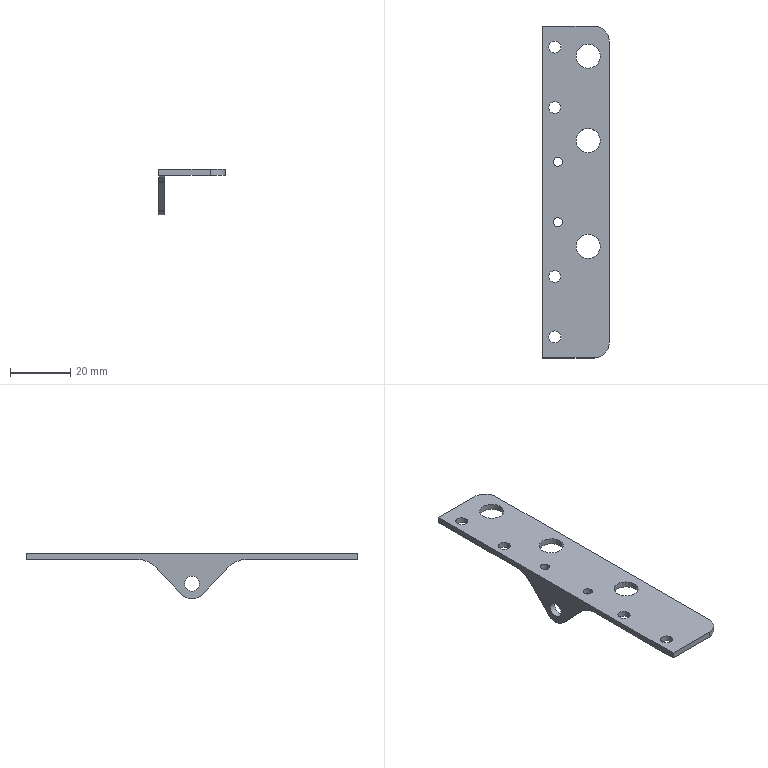Part | STEP file | 1-28.4 | 1 solid | 24 faces | box 22 x 110 x 15 mm | volume 4787 mm3 | cylinder 15 | plane 9 | commonest cylinder face diameters 4 x4 8 x3 10 x3 3 x2 16 x2 5 x1